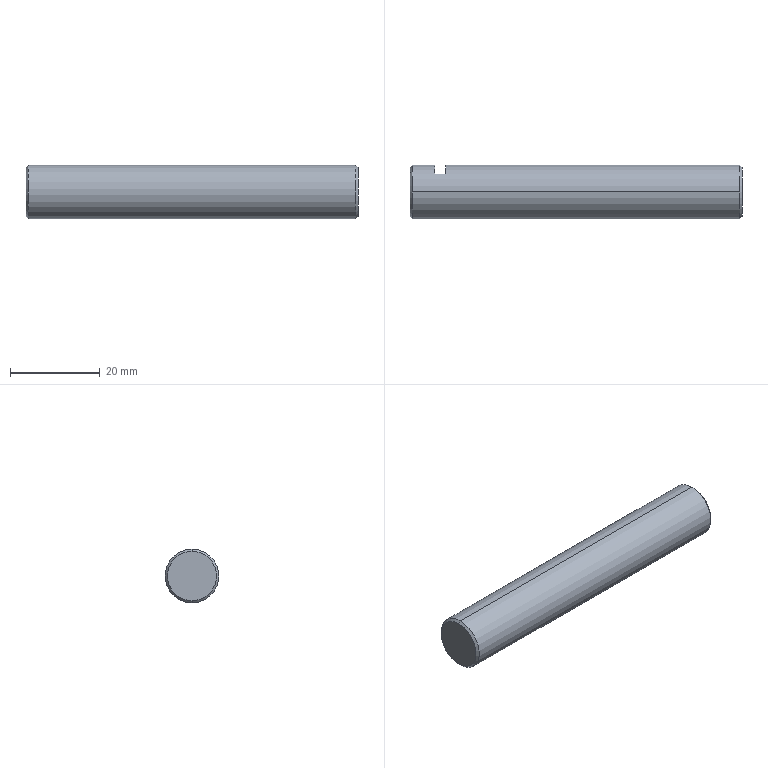Part | STEP file | 0245_010_PCLKG12-74 | 1 solid | 11 faces | box 74 x 12 x 12 mm | volume 8329 mm3 | plane 5 | cone 4 | cylinder 2 | commonest cylinder face diameters 12 x2
STEP:
#1=CARTESIAN_POINT('',(0.,0.,0.));
#2=DIRECTION('',(0.,0.,1.));
#3=DIRECTION('',(1.,0.,0.));
#4=AXIS2_PLACEMENT_3D('',#1,#2,#3);
#5=CARTESIAN_POINT('',(5.5,4.,-4.472));
#6=VERTEX_POINT('',#5);
#7=CARTESIAN_POINT('',(8.,4.,-4.472));
#8=VERTEX_POINT('',#7);
#9=CARTESIAN_POINT('',(37.,4.,-4.472));
#10=DIRECTION('',(1.,0.,0.));
#11=VECTOR('',#10,1.);
#12=LINE('',#9,#11);
#13=CARTESIAN_POINT('',(37.,0.,0.));
#14=DIRECTION('',(1.,0.,0.));
#15=DIRECTION('',(0.,0.,-1.));
#16=AXIS2_PLACEMENT_3D('',#13,#14,#15);
#17=CYLINDRICAL_SURFACE('',#16,6.);
#18=CARTESIAN_POINT('',(0.7297,0.));
#19=DIRECTION('',(0.,1.));
#20=VECTOR('',#19,1.);
#21=LINE('',#18,#20);
#22=(GEOMETRIC_REPRESENTATION_CONTEXT(2)PARAMETRIC_REPRESENTATION_CONTEXT()REPRESENTATION_CONTEXT('',''));
#23=DEFINITIONAL_REPRESENTATION('',(#21),#22);
#24=PCURVE('',#17,#23);
#25=CARTESIAN_POINT('',(5.5,4.,12.));
#26=DIRECTION('',(0.,-1.,0.));
#27=DIRECTION('',(0.,0.,-1.));
#28=AXIS2_PLACEMENT_3D('',#25,#26,#27);
#29=PLANE('',#28);
#30=CARTESIAN_POINT('',(16.472,31.5));
#31=DIRECTION('',(0.,1.));
#32=VECTOR('',#31,1.);
#33=LINE('',#30,#32);
#34=(GEOMETRIC_REPRESENTATION_CONTEXT(2)PARAMETRIC_REPRESENTATION_CONTEXT()REPRESENTATION_CONTEXT('',''));
#35=DEFINITIONAL_REPRESENTATION('',(#33),#34);
#36=PCURVE('',#29,#35);
#37=SURFACE_CURVE('',#12,(#24,#36),.PCURVE_S1.);
#38=EDGE_CURVE('',#6,#8,#37,.T.);
#39=ORIENTED_EDGE('',*,*,#38,.T.);
#40=CARTESIAN_POINT('',(8.,4.,4.472));
#41=VERTEX_POINT('',#40);
#42=CARTESIAN_POINT('',(8.,0.,0.));
#43=DIRECTION('',(1.,0.,0.));
#44=DIRECTION('',(0.,0.,-1.));
#45=AXIS2_PLACEMENT_3D('',#42,#43,#44);
#46=CIRCLE('',#45,6.);
#47=CARTESIAN_POINT('',(0.,-29.));
#48=DIRECTION('',(1.,0.));
#49=VECTOR('',#48,1.);
#50=LINE('',#47,#49);
#51=(GEOMETRIC_REPRESENTATION_CONTEXT(2)PARAMETRIC_REPRESENTATION_CONTEXT()REPRESENTATION_CONTEXT('',''));
#52=DEFINITIONAL_REPRESENTATION('',(#50),#51);
#53=PCURVE('',#17,#52);
#54=CARTESIAN_POINT('',(8.,4.,12.));
#55=DIRECTION('',(1.,0.,0.));
#56=DIRECTION('',(0.,0.,-1.));
#57=AXIS2_PLACEMENT_3D('',#54,#55,#56);
#58=PLANE('',#57);
#59=CARTESIAN_POINT('',(12.,-4.));
#60=DIRECTION('',(1.,0.));
#61=AXIS2_PLACEMENT_2D('',#59,#60);
#62=CIRCLE('',#61,6.);
#63=(GEOMETRIC_REPRESENTATION_CONTEXT(2)PARAMETRIC_REPRESENTATION_CONTEXT()REPRESENTATION_CONTEXT('',''));
#64=DEFINITIONAL_REPRESENTATION('',(#62),#63);
#65=PCURVE('',#58,#64);
#66=SURFACE_CURVE('',#46,(#53,#65),.PCURVE_S1.);
#67=EDGE_CURVE('',#8,#41,#66,.T.);
#68=ORIENTED_EDGE('',*,*,#67,.T.);
#69=CARTESIAN_POINT('',(5.5,4.,4.472));
#70=VERTEX_POINT('',#69);
#71=CARTESIAN_POINT('',(5.5,4.,4.472));
#72=DIRECTION('',(-1.,0.,0.));
#73=VECTOR('',#72,1.);
#74=LINE('',#71,#73);
#75=CARTESIAN_POINT('',(2.412,-31.5));
#76=DIRECTION('',(0.,-1.));
#77=VECTOR('',#76,1.);
#78=LINE('',#75,#77);
#79=(GEOMETRIC_REPRESENTATION_CONTEXT(2)PARAMETRIC_REPRESENTATION_CONTEXT()REPRESENTATION_CONTEXT('',''));
#80=DEFINITIONAL_REPRESENTATION('',(#78),#79);
#81=PCURVE('',#17,#80);
#82=CARTESIAN_POINT('',(7.528,0.));
#83=DIRECTION('',(0.,-1.));
#84=VECTOR('',#83,1.);
#85=LINE('',#82,#84);
#86=(GEOMETRIC_REPRESENTATION_CONTEXT(2)PARAMETRIC_REPRESENTATION_CONTEXT()REPRESENTATION_CONTEXT('',''));
#87=DEFINITIONAL_REPRESENTATION('',(#85),#86);
#88=PCURVE('',#29,#87);
#89=SURFACE_CURVE('',#74,(#81,#88),.PCURVE_S1.);
#90=EDGE_CURVE('',#41,#70,#89,.T.);
#91=ORIENTED_EDGE('',*,*,#90,.T.);
#92=CARTESIAN_POINT('',(5.5,0.,0.));
#93=DIRECTION('',(-1.,0.,0.));
#94=DIRECTION('',(0.,0.,-1.));
#95=AXIS2_PLACEMENT_3D('',#92,#93,#94);
#96=CIRCLE('',#95,6.);
#97=CARTESIAN_POINT('',(6.283,-31.5));
#98=DIRECTION('',(-1.,0.));
#99=VECTOR('',#98,1.);
#100=LINE('',#97,#99);
#101=(GEOMETRIC_REPRESENTATION_CONTEXT(2)PARAMETRIC_REPRESENTATION_CONTEXT()REPRESENTATION_CONTEXT('',''));
#102=DEFINITIONAL_REPRESENTATION('',(#100),#101);
#103=PCURVE('',#17,#102);
#104=CARTESIAN_POINT('',(5.5,8.,12.));
#105=DIRECTION('',(-1.,0.,0.));
#106=DIRECTION('',(0.,0.,1.));
#107=AXIS2_PLACEMENT_3D('',#104,#105,#106);
#108=PLANE('',#107);
#109=CARTESIAN_POINT('',(-12.,-8.));
#110=DIRECTION('',(-1.,0.));
#111=AXIS2_PLACEMENT_2D('',#109,#110);
#112=CIRCLE('',#111,6.);
#113=(GEOMETRIC_REPRESENTATION_CONTEXT(2)PARAMETRIC_REPRESENTATION_CONTEXT()REPRESENTATION_CONTEXT('',''));
#114=DEFINITIONAL_REPRESENTATION('',(#112),#113);
#115=PCURVE('',#108,#114);
#116=SURFACE_CURVE('',#96,(#103,#115),.PCURVE_S1.);
#117=EDGE_CURVE('',#70,#6,#116,.T.);
#118=ORIENTED_EDGE('',*,*,#117,.T.);
#119=EDGE_LOOP('',(#39,#68,#91,#118));
#120=FACE_BOUND('',#119,.T.);
#121=CARTESIAN_POINT('',(0.5,0.,-6.));
#122=VERTEX_POINT('',#121);
#123=CARTESIAN_POINT('',(0.5,0.,6.));
#124=VERTEX_POINT('',#123);
#125=CARTESIAN_POINT('',(0.5,0.,0.));
#126=DIRECTION('',(1.,0.,0.));
#127=DIRECTION('',(0.,0.,-1.));
#128=AXIS2_PLACEMENT_3D('',#125,#126,#127);
#129=CIRCLE('',#128,6.);
#130=CARTESIAN_POINT('',(0.,-36.5));
#131=DIRECTION('',(1.,0.));
#132=VECTOR('',#131,1.);
#133=LINE('',#130,#132);
#134=(GEOMETRIC_REPRESENTATION_CONTEXT(2)PARAMETRIC_REPRESENTATION_CONTEXT()REPRESENTATION_CONTEXT('',''));
#135=DEFINITIONAL_REPRESENTATION('',(#133),#134);
#136=PCURVE('',#17,#135);
#137=CARTESIAN_POINT('',(0.5,0.,0.));
#138=DIRECTION('',(1.,0.,0.));
#139=DIRECTION('',(0.,0.,-1.));
#140=AXIS2_PLACEMENT_3D('',#137,#138,#139);
#141=CONICAL_SURFACE('',#140,6.,0.7854);
#142=CARTESIAN_POINT('',(0.,0.));
#143=DIRECTION('',(1.,0.));
#144=VECTOR('',#143,1.);
#145=LINE('',#142,#144);
#146=(GEOMETRIC_REPRESENTATION_CONTEXT(2)PARAMETRIC_REPRESENTATION_CONTEXT()REPRESENTATION_CONTEXT('',''));
#147=DEFINITIONAL_REPRESENTATION('',(#145),#146);
#148=PCURVE('',#141,#147);
#149=SURFACE_CURVE('',#129,(#136,#148),.PCURVE_S1.);
#150=EDGE_CURVE('',#122,#124,#149,.T.);
#151=ORIENTED_EDGE('',*,*,#150,.T.);
#152=CARTESIAN_POINT('',(73.5,0.,6.));
#153=VERTEX_POINT('',#152);
#154=CARTESIAN_POINT('',(37.,0.,6.));
#155=DIRECTION('',(1.,0.,0.));
#156=VECTOR('',#155,1.);
#157=LINE('',#154,#156);
#158=CARTESIAN_POINT('',(3.142,0.));
#159=DIRECTION('',(0.,1.));
#160=VECTOR('',#159,1.);
#161=LINE('',#158,#160);
#162=(GEOMETRIC_REPRESENTATION_CONTEXT(2)PARAMETRIC_REPRESENTATION_CONTEXT()REPRESENTATION_CONTEXT('',''));
#163=DEFINITIONAL_REPRESENTATION('',(#161),#162);
#164=PCURVE('',#17,#163);
#165=CARTESIAN_POINT('',(37.,0.,0.));
#166=DIRECTION('',(1.,0.,0.));
#167=DIRECTION('',(0.,0.,-1.));
#168=AXIS2_PLACEMENT_3D('',#165,#166,#167);
#169=CYLINDRICAL_SURFACE('',#168,6.);
#170=CARTESIAN_POINT('',(3.142,0.));
#171=DIRECTION('',(0.,1.));
#172=VECTOR('',#171,1.);
#173=LINE('',#170,#172);
#174=(GEOMETRIC_REPRESENTATION_CONTEXT(2)PARAMETRIC_REPRESENTATION_CONTEXT()REPRESENTATION_CONTEXT('',''));
#175=DEFINITIONAL_REPRESENTATION('',(#173),#174);
#176=PCURVE('',#169,#175);
#177=SURFACE_CURVE('',#157,(#164,#176),.PCURVE_S1.);
#178=EDGE_CURVE('',#124,#153,#177,.T.);
#179=ORIENTED_EDGE('',*,*,#178,.T.);
#180=CARTESIAN_POINT('',(73.5,0.,-6.));
#181=VERTEX_POINT('',#180);
#182=CARTESIAN_POINT('',(73.5,0.,0.));
#183=DIRECTION('',(-1.,0.,0.));
#184=DIRECTION('',(0.,0.,-1.));
#185=AXIS2_PLACEMENT_3D('',#182,#183,#184);
#186=CIRCLE('',#185,6.);
#187=CARTESIAN_POINT('',(6.283,36.5));
#188=DIRECTION('',(-1.,0.));
#189=VECTOR('',#188,1.);
#190=LINE('',#187,#189);
#191=(GEOMETRIC_REPRESENTATION_CONTEXT(2)PARAMETRIC_REPRESENTATION_CONTEXT()REPRESENTATION_CONTEXT('',''));
#192=DEFINITIONAL_REPRESENTATION('',(#190),#191);
#193=PCURVE('',#17,#192);
#194=CARTESIAN_POINT('',(73.5,0.,0.));
#195=DIRECTION('',(-1.,0.,0.));
#196=DIRECTION('',(0.,0.,1.));
#197=AXIS2_PLACEMENT_3D('',#194,#195,#196);
#198=CONICAL_SURFACE('',#197,6.,0.7854);
#199=CARTESIAN_POINT('',(-3.142,0.));
#200=DIRECTION('',(1.,0.));
#201=VECTOR('',#200,1.);
#202=LINE('',#199,#201);
#203=(GEOMETRIC_REPRESENTATION_CONTEXT(2)PARAMETRIC_REPRESENTATION_CONTEXT()REPRESENTATION_CONTEXT('',''));
#204=DEFINITIONAL_REPRESENTATION('',(#202),#203);
#205=PCURVE('',#198,#204);
#206=SURFACE_CURVE('',#186,(#193,#205),.PCURVE_S1.);
#207=EDGE_CURVE('',#153,#181,#206,.T.);
#208=ORIENTED_EDGE('',*,*,#207,.T.);
#209=CARTESIAN_POINT('',(37.,0.,-6.));
#210=DIRECTION('',(1.,0.,0.));
#211=VECTOR('',#210,1.);
#212=LINE('',#209,#211);
#213=CARTESIAN_POINT('',(0.,0.));
#214=DIRECTION('',(0.,1.));
#215=VECTOR('',#214,1.);
#216=LINE('',#213,#215);
#217=(GEOMETRIC_REPRESENTATION_CONTEXT(2)PARAMETRIC_REPRESENTATION_CONTEXT()REPRESENTATION_CONTEXT('',''));
#218=DEFINITIONAL_REPRESENTATION('',(#216),#217);
#219=PCURVE('',#17,#218);
#220=CARTESIAN_POINT('',(6.283,0.));
#221=DIRECTION('',(0.,1.));
#222=VECTOR('',#221,1.);
#223=LINE('',#220,#222);
#224=(GEOMETRIC_REPRESENTATION_CONTEXT(2)PARAMETRIC_REPRESENTATION_CONTEXT()REPRESENTATION_CONTEXT('',''));
#225=DEFINITIONAL_REPRESENTATION('',(#223),#224);
#226=PCURVE('',#169,#225);
#227=SURFACE_CURVE('',#212,(#219,#226),.PCURVE_S1.);
#228=EDGE_CURVE('',#122,#181,#227,.T.);
#229=ORIENTED_EDGE('',*,*,#228,.F.);
#230=EDGE_LOOP('',(#151,#179,#208,#229));
#231=FACE_BOUND('',#230,.T.);
#232=ADVANCED_FACE('',(#120,#231),#17,.T.);
#233=CARTESIAN_POINT('',(0.,0.,-5.5));
#234=VERTEX_POINT('',#233);
#235=CARTESIAN_POINT('',(0.,0.,5.5));
#236=VERTEX_POINT('',#235);
#237=CARTESIAN_POINT('',(0.,0.,0.));
#238=DIRECTION('',(1.,0.,0.));
#239=DIRECTION('',(0.,0.,-1.));
#240=AXIS2_PLACEMENT_3D('',#237,#238,#239);
#241=CIRCLE('',#240,5.5);
#242=CARTESIAN_POINT('',(0.,-0.5));
#243=DIRECTION('',(1.,0.));
#244=VECTOR('',#243,1.);
#245=LINE('',#242,#244);
#246=(GEOMETRIC_REPRESENTATION_CONTEXT(2)PARAMETRIC_REPRESENTATION_CONTEXT()REPRESENTATION_CONTEXT('',''));
#247=DEFINITIONAL_REPRESENTATION('',(#245),#246);
#248=PCURVE('',#141,#247);
#249=CARTESIAN_POINT('',(0.,2.75,0.));
#250=DIRECTION('',(-1.,0.,0.));
#251=DIRECTION('',(0.,0.,1.));
#252=AXIS2_PLACEMENT_3D('',#249,#250,#251);
#253=PLANE('',#252);
#254=CARTESIAN_POINT('',(-5.5,-2.75));
#255=CARTESIAN_POINT('',(-5.5,6.776));
#256=CARTESIAN_POINT('',(2.75,2.013));
#257=CARTESIAN_POINT('',(11.,-2.75));
#258=CARTESIAN_POINT('',(2.75,-7.513));
#259=CARTESIAN_POINT('',(-5.5,-12.276));
#260=CARTESIAN_POINT('',(-5.5,-2.75));
#261=(BOUNDED_CURVE()B_SPLINE_CURVE(2,(#254,#255,#256,#257,#258,#259,#260),.UNSPECIFIED.,.T.,.F.)B_SPLINE_CURVE_WITH_KNOTS((1,2,2,2,2,1),(-2.094,0.,2.094,4.189,6.283,8.378),.UNSPECIFIED.)CURVE()GEOMETRIC_REPRESENTATION_ITEM()RATIONAL_B_SPLINE_CURVE((1.,0.5,1.,0.5,1.,0.5,1.))REPRESENTATION_ITEM(''));
#262=(GEOMETRIC_REPRESENTATION_CONTEXT(2)PARAMETRIC_REPRESENTATION_CONTEXT()REPRESENTATION_CONTEXT('',''));
#263=DEFINITIONAL_REPRESENTATION('',(#261),#262);
#264=PCURVE('',#253,#263);
#265=SURFACE_CURVE('',#241,(#248,#264),.PCURVE_S1.);
#266=EDGE_CURVE('',#234,#236,#265,.T.);
#267=ORIENTED_EDGE('',*,*,#266,.T.);
#268=CARTESIAN_POINT('',(0.5,0.,6.));
#269=DIRECTION('',(0.7071,0.,0.7071));
#270=VECTOR('',#269,1.);
#271=LINE('',#268,#270);
#272=CARTESIAN_POINT('',(3.142,0.));
#273=DIRECTION('',(0.,1.));
#274=VECTOR('',#273,1.);
#275=LINE('',#272,#274);
#276=(GEOMETRIC_REPRESENTATION_CONTEXT(2)PARAMETRIC_REPRESENTATION_CONTEXT()REPRESENTATION_CONTEXT('',''));
#277=DEFINITIONAL_REPRESENTATION('',(#275),#276);
#278=PCURVE('',#141,#277);
#279=CARTESIAN_POINT('',(0.5,0.,0.));
#280=DIRECTION('',(1.,0.,0.));
#281=DIRECTION('',(0.,0.,-1.));
#282=AXIS2_PLACEMENT_3D('',#279,#280,#281);
#283=CONICAL_SURFACE('',#282,6.,0.7854);
#284=CARTESIAN_POINT('',(3.142,0.));
#285=DIRECTION('',(0.,1.));
#286=VECTOR('',#285,1.);
#287=LINE('',#284,#286);
#288=(GEOMETRIC_REPRESENTATION_CONTEXT(2)PARAMETRIC_REPRESENTATION_CONTEXT()REPRESENTATION_CONTEXT('',''));
#289=DEFINITIONAL_REPRESENTATION('',(#287),#288);
#290=PCURVE('',#283,#289);
#291=SURFACE_CURVE('',#271,(#278,#290),.PCURVE_S1.);
#292=EDGE_CURVE('',#236,#124,#291,.T.);
#293=ORIENTED_EDGE('',*,*,#292,.T.);
#294=ORIENTED_EDGE('',*,*,#150,.F.);
#295=CARTESIAN_POINT('',(0.5,0.,-6.));
#296=DIRECTION('',(0.7071,0.,-0.7071));
#297=VECTOR('',#296,1.);
#298=LINE('',#295,#297);
#299=CARTESIAN_POINT('',(0.,0.));
#300=DIRECTION('',(0.,1.));
#301=VECTOR('',#300,1.);
#302=LINE('',#299,#301);
#303=(GEOMETRIC_REPRESENTATION_CONTEXT(2)PARAMETRIC_REPRESENTATION_CONTEXT()REPRESENTATION_CONTEXT('',''));
#304=DEFINITIONAL_REPRESENTATION('',(#302),#303);
#305=PCURVE('',#141,#304);
#306=CARTESIAN_POINT('',(6.283,0.));
#307=DIRECTION('',(0.,1.));
#308=VECTOR('',#307,1.);
#309=LINE('',#306,#308);
#310=(GEOMETRIC_REPRESENTATION_CONTEXT(2)PARAMETRIC_REPRESENTATION_CONTEXT()REPRESENTATION_CONTEXT('',''));
#311=DEFINITIONAL_REPRESENTATION('',(#309),#310);
#312=PCURVE('',#283,#311);
#313=SURFACE_CURVE('',#298,(#305,#312),.PCURVE_S1.);
#314=EDGE_CURVE('',#234,#122,#313,.T.);
#315=ORIENTED_EDGE('',*,*,#314,.F.);
#316=EDGE_LOOP('',(#267,#293,#294,#315));
#317=FACE_BOUND('',#316,.T.);
#318=ADVANCED_FACE('',(#317),#141,.T.);
#319=CARTESIAN_POINT('',(74.,0.,5.5));
#320=VERTEX_POINT('',#319);
#321=CARTESIAN_POINT('',(74.,0.,-5.5));
#322=VERTEX_POINT('',#321);
#323=CARTESIAN_POINT('',(74.,0.,0.));
#324=DIRECTION('',(-1.,0.,0.));
#325=DIRECTION('',(0.,0.,1.));
#326=AXIS2_PLACEMENT_3D('',#323,#324,#325);
#327=CIRCLE('',#326,5.5);
#328=CARTESIAN_POINT('',(0.,-0.5));
#329=DIRECTION('',(1.,0.));
#330=VECTOR('',#329,1.);
#331=LINE('',#328,#330);
#332=(GEOMETRIC_REPRESENTATION_CONTEXT(2)PARAMETRIC_REPRESENTATION_CONTEXT()REPRESENTATION_CONTEXT('',''));
#333=DEFINITIONAL_REPRESENTATION('',(#331),#332);
#334=PCURVE('',#198,#333);
#335=CARTESIAN_POINT('',(74.,2.75,0.));
#336=DIRECTION('',(1.,0.,0.));
#337=DIRECTION('',(0.,0.,-1.));
#338=AXIS2_PLACEMENT_3D('',#335,#336,#337);
#339=PLANE('',#338);
#340=CARTESIAN_POINT('',(-5.5,-2.75));
#341=CARTESIAN_POINT('',(-5.5,6.776));
#342=CARTESIAN_POINT('',(2.75,2.013));
#343=CARTESIAN_POINT('',(11.,-2.75));
#344=CARTESIAN_POINT('',(2.75,-7.513));
#345=CARTESIAN_POINT('',(-5.5,-12.276));
#346=CARTESIAN_POINT('',(-5.5,-2.75));
#347=(BOUNDED_CURVE()B_SPLINE_CURVE(2,(#340,#341,#342,#343,#344,#345,#346),.UNSPECIFIED.,.T.,.F.)B_SPLINE_CURVE_WITH_KNOTS((1,2,2,2,2,1),(-2.094,0.,2.094,4.189,6.283,8.378),.UNSPECIFIED.)CURVE()GEOMETRIC_REPRESENTATION_ITEM()RATIONAL_B_SPLINE_CURVE((1.,0.5,1.,0.5,1.,0.5,1.))REPRESENTATION_ITEM(''));
#348=(GEOMETRIC_REPRESENTATION_CONTEXT(2)PARAMETRIC_REPRESENTATION_CONTEXT()REPRESENTATION_CONTEXT('',''));
#349=DEFINITIONAL_REPRESENTATION('',(#347),#348);
#350=PCURVE('',#339,#349);
#351=SURFACE_CURVE('',#327,(#334,#350),.PCURVE_S1.);
#352=EDGE_CURVE('',#320,#322,#351,.T.);
#353=ORIENTED_EDGE('',*,*,#352,.T.);
#354=CARTESIAN_POINT('',(73.5,0.,-6.));
#355=DIRECTION('',(-0.7071,0.,-0.7071));
#356=VECTOR('',#355,1.);
#357=LINE('',#354,#356);
#358=CARTESIAN_POINT('',(3.142,0.));
#359=DIRECTION('',(0.,1.));
#360=VECTOR('',#359,1.);
#361=LINE('',#358,#360);
#362=(GEOMETRIC_REPRESENTATION_CONTEXT(2)PARAMETRIC_REPRESENTATION_CONTEXT()REPRESENTATION_CONTEXT('',''));
#363=DEFINITIONAL_REPRESENTATION('',(#361),#362);
#364=PCURVE('',#198,#363);
#365=CARTESIAN_POINT('',(73.5,0.,0.));
#366=DIRECTION('',(-1.,0.,0.));
#367=DIRECTION('',(0.,0.,1.));
#368=AXIS2_PLACEMENT_3D('',#365,#366,#367);
#369=CONICAL_SURFACE('',#368,6.,0.7854);
#370=CARTESIAN_POINT('',(3.142,0.));
#371=DIRECTION('',(0.,1.));
#372=VECTOR('',#371,1.);
#373=LINE('',#370,#372);
#374=(GEOMETRIC_REPRESENTATION_CONTEXT(2)PARAMETRIC_REPRESENTATION_CONTEXT()REPRESENTATION_CONTEXT('',''));
#375=DEFINITIONAL_REPRESENTATION('',(#373),#374);
#376=PCURVE('',#369,#375);
#377=SURFACE_CURVE('',#357,(#364,#376),.PCURVE_S1.);
#378=EDGE_CURVE('',#322,#181,#377,.T.);
#379=ORIENTED_EDGE('',*,*,#378,.T.);
#380=ORIENTED_EDGE('',*,*,#207,.F.);
#381=CARTESIAN_POINT('',(73.5,0.,6.));
#382=DIRECTION('',(-0.7071,0.,0.7071));
#383=VECTOR('',#382,1.);
#384=LINE('',#381,#383);
#385=CARTESIAN_POINT('',(0.,0.));
#386=DIRECTION('',(0.,1.));
#387=VECTOR('',#386,1.);
#388=LINE('',#385,#387);
#389=(GEOMETRIC_REPRESENTATION_CONTEXT(2)PARAMETRIC_REPRESENTATION_CONTEXT()REPRESENTATION_CONTEXT('',''));
#390=DEFINITIONAL_REPRESENTATION('',(#388),#389);
#391=PCURVE('',#198,#390);
#392=CARTESIAN_POINT('',(6.283,0.));
#393=DIRECTION('',(0.,1.));
#394=VECTOR('',#393,1.);
#395=LINE('',#392,#394);
#396=(GEOMETRIC_REPRESENTATION_CONTEXT(2)PARAMETRIC_REPRESENTATION_CONTEXT()REPRESENTATION_CONTEXT('',''));
#397=DEFINITIONAL_REPRESENTATION('',(#395),#396);
#398=PCURVE('',#369,#397);
#399=SURFACE_CURVE('',#384,(#391,#398),.PCURVE_S1.);
#400=EDGE_CURVE('',#320,#153,#399,.T.);
#401=ORIENTED_EDGE('',*,*,#400,.F.);
#402=EDGE_LOOP('',(#353,#379,#380,#401));
#403=FACE_BOUND('',#402,.T.);
#404=ADVANCED_FACE('',(#403),#198,.T.);
#405=ORIENTED_EDGE('',*,*,#178,.F.);
#406=CARTESIAN_POINT('',(0.5,0.,0.));
#407=DIRECTION('',(1.,0.,0.));
#408=DIRECTION('',(0.,0.,-1.));
#409=AXIS2_PLACEMENT_3D('',#406,#407,#408);
#410=CIRCLE('',#409,6.);
#411=CARTESIAN_POINT('',(0.,-36.5));
#412=DIRECTION('',(1.,0.));
#413=VECTOR('',#412,1.);
#414=LINE('',#411,#413);
#415=(GEOMETRIC_REPRESENTATION_CONTEXT(2)PARAMETRIC_REPRESENTATION_CONTEXT()REPRESENTATION_CONTEXT('',''));
#416=DEFINITIONAL_REPRESENTATION('',(#414),#415);
#417=PCURVE('',#169,#416);
#418=CARTESIAN_POINT('',(0.,0.));
#419=DIRECTION('',(1.,0.));
#420=VECTOR('',#419,1.);
#421=LINE('',#418,#420);
#422=(GEOMETRIC_REPRESENTATION_CONTEXT(2)PARAMETRIC_REPRESENTATION_CONTEXT()REPRESENTATION_CONTEXT('',''));
#423=DEFINITIONAL_REPRESENTATION('',(#421),#422);
#424=PCURVE('',#283,#423);
#425=SURFACE_CURVE('',#410,(#417,#424),.PCURVE_S1.);
#426=EDGE_CURVE('',#124,#122,#425,.T.);
#427=ORIENTED_EDGE('',*,*,#426,.T.);
#428=ORIENTED_EDGE('',*,*,#228,.T.);
#429=CARTESIAN_POINT('',(73.5,0.,0.));
#430=DIRECTION('',(-1.,0.,0.));
#431=DIRECTION('',(0.,0.,-1.));
#432=AXIS2_PLACEMENT_3D('',#429,#430,#431);
#433=CIRCLE('',#432,6.);
#434=CARTESIAN_POINT('',(6.283,36.5));
#435=DIRECTION('',(-1.,0.));
#436=VECTOR('',#435,1.);
#437=LINE('',#434,#436);
#438=(GEOMETRIC_REPRESENTATION_CONTEXT(2)PARAMETRIC_REPRESENTATION_CONTEXT()REPRESENTATION_CONTEXT('',''));
#439=DEFINITIONAL_REPRESENTATION('',(#437),#438);
#440=PCURVE('',#169,#439);
#441=CARTESIAN_POINT('',(3.142,0.));
#442=DIRECTION('',(1.,0.));
#443=VECTOR('',#442,1.);
#444=LINE('',#441,#443);
#445=(GEOMETRIC_REPRESENTATION_CONTEXT(2)PARAMETRIC_REPRESENTATION_CONTEXT()REPRESENTATION_CONTEXT('',''));
#446=DEFINITIONAL_REPRESENTATION('',(#444),#445);
#447=PCURVE('',#369,#446);
#448=SURFACE_CURVE('',#433,(#440,#447),.PCURVE_S1.);
#449=EDGE_CURVE('',#181,#153,#448,.T.);
#450=ORIENTED_EDGE('',*,*,#449,.T.);
#451=EDGE_LOOP('',(#405,#427,#428,#450));
#452=FACE_BOUND('',#451,.T.);
#453=ADVANCED_FACE('',(#452),#169,.T.);
#454=CARTESIAN_POINT('',(8.,4.,12.));
#455=DIRECTION('',(0.,0.,-1.));
#456=VECTOR('',#455,1.);
#457=LINE('',#454,#456);
#458=CARTESIAN_POINT('',(0.,0.));
#459=DIRECTION('',(1.,0.));
#460=VECTOR('',#459,1.);
#461=LINE('',#458,#460);
#462=(GEOMETRIC_REPRESENTATION_CONTEXT(2)PARAMETRIC_REPRESENTATION_CONTEXT()REPRESENTATION_CONTEXT('',''));
#463=DEFINITIONAL_REPRESENTATION('',(#461),#462);
#464=PCURVE('',#58,#463);
#465=CARTESIAN_POINT('',(0.,2.5));
#466=DIRECTION('',(1.,0.));
#467=VECTOR('',#466,1.);
#468=LINE('',#465,#467);
#469=(GEOMETRIC_REPRESENTATION_CONTEXT(2)PARAMETRIC_REPRESENTATION_CONTEXT()REPRESENTATION_CONTEXT('',''));
#470=DEFINITIONAL_REPRESENTATION('',(#468),#469);
#471=PCURVE('',#29,#470);
#472=SURFACE_CURVE('',#457,(#464,#471),.PCURVE_S1.);
#473=EDGE_CURVE('',#41,#8,#472,.T.);
#474=ORIENTED_EDGE('',*,*,#473,.F.);
#475=ORIENTED_EDGE('',*,*,#67,.F.);
#476=EDGE_LOOP('',(#474,#475));
#477=FACE_BOUND('',#476,.T.);
#478=ADVANCED_FACE('',(#477),#58,.F.);
#479=CARTESIAN_POINT('',(5.5,4.,12.));
#480=DIRECTION('',(0.,0.,-1.));
#481=VECTOR('',#480,1.);
#482=LINE('',#479,#481);
#483=CARTESIAN_POINT('',(0.,0.));
#484=DIRECTION('',(1.,0.));
#485=VECTOR('',#484,1.);
#486=LINE('',#483,#485);
#487=(GEOMETRIC_REPRESENTATION_CONTEXT(2)PARAMETRIC_REPRESENTATION_CONTEXT()REPRESENTATION_CONTEXT('',''));
#488=DEFINITIONAL_REPRESENTATION('',(#486),#487);
#489=PCURVE('',#29,#488);
#490=CARTESIAN_POINT('',(0.,-4.));
#491=DIRECTION('',(-1.,0.));
#492=VECTOR('',#491,1.);
#493=LINE('',#490,#492);
#494=(GEOMETRIC_REPRESENTATION_CONTEXT(2)PARAMETRIC_REPRESENTATION_CONTEXT()REPRESENTATION_CONTEXT('',''));
#495=DEFINITIONAL_REPRESENTATION('',(#493),#494);
#496=PCURVE('',#108,#495);
#497=SURFACE_CURVE('',#482,(#489,#496),.PCURVE_S1.);
#498=EDGE_CURVE('',#70,#6,#497,.T.);
#499=ORIENTED_EDGE('',*,*,#498,.F.);
#500=ORIENTED_EDGE('',*,*,#90,.F.);
#501=ORIENTED_EDGE('',*,*,#473,.T.);
#502=ORIENTED_EDGE('',*,*,#38,.F.);
#503=EDGE_LOOP('',(#499,#500,#501,#502));
#504=FACE_BOUND('',#503,.T.);
#505=ADVANCED_FACE('',(#504),#29,.F.);
#506=ORIENTED_EDGE('',*,*,#498,.T.);
#507=ORIENTED_EDGE('',*,*,#117,.F.);
#508=EDGE_LOOP('',(#506,#507));
#509=FACE_BOUND('',#508,.T.);
#510=ADVANCED_FACE('',(#509),#108,.F.);
#511=ORIENTED_EDGE('',*,*,#292,.F.);
#512=CARTESIAN_POINT('',(0.,0.,0.));
#513=DIRECTION('',(1.,0.,0.));
#514=DIRECTION('',(0.,0.,-1.));
#515=AXIS2_PLACEMENT_3D('',#512,#513,#514);
#516=CIRCLE('',#515,5.5);
#517=CARTESIAN_POINT('',(0.,-0.5));
#518=DIRECTION('',(1.,0.));
#519=VECTOR('',#518,1.);
#520=LINE('',#517,#519);
#521=(GEOMETRIC_REPRESENTATION_CONTEXT(2)PARAMETRIC_REPRESENTATION_CONTEXT()REPRESENTATION_CONTEXT('',''));
#522=DEFINITIONAL_REPRESENTATION('',(#520),#521);
#523=PCURVE('',#283,#522);
#524=CARTESIAN_POINT('',(-5.5,-2.75));
#525=CARTESIAN_POINT('',(-5.5,6.776));
#526=CARTESIAN_POINT('',(2.75,2.013));
#527=CARTESIAN_POINT('',(11.,-2.75));
#528=CARTESIAN_POINT('',(2.75,-7.513));
#529=CARTESIAN_POINT('',(-5.5,-12.276));
#530=CARTESIAN_POINT('',(-5.5,-2.75));
#531=(BOUNDED_CURVE()B_SPLINE_CURVE(2,(#524,#525,#526,#527,#528,#529,#530),.UNSPECIFIED.,.T.,.F.)B_SPLINE_CURVE_WITH_KNOTS((1,2,2,2,2,1),(-2.094,0.,2.094,4.189,6.283,8.378),.UNSPECIFIED.)CURVE()GEOMETRIC_REPRESENTATION_ITEM()RATIONAL_B_SPLINE_CURVE((1.,0.5,1.,0.5,1.,0.5,1.))REPRESENTATION_ITEM(''));
#532=(GEOMETRIC_REPRESENTATION_CONTEXT(2)PARAMETRIC_REPRESENTATION_CONTEXT()REPRESENTATION_CONTEXT('',''));
#533=DEFINITIONAL_REPRESENTATION('',(#531),#532);
#534=PCURVE('',#253,#533);
#535=SURFACE_CURVE('',#516,(#523,#534),.PCURVE_S1.);
#536=EDGE_CURVE('',#236,#234,#535,.T.);
#537=ORIENTED_EDGE('',*,*,#536,.T.);
#538=ORIENTED_EDGE('',*,*,#314,.T.);
#539=ORIENTED_EDGE('',*,*,#426,.F.);
#540=EDGE_LOOP('',(#511,#537,#538,#539));
#541=FACE_BOUND('',#540,.T.);
#542=ADVANCED_FACE('',(#541),#283,.T.);
#543=ORIENTED_EDGE('',*,*,#378,.F.);
#544=CARTESIAN_POINT('',(74.,0.,0.));
#545=DIRECTION('',(-1.,0.,0.));
#546=DIRECTION('',(0.,0.,1.));
#547=AXIS2_PLACEMENT_3D('',#544,#545,#546);
#548=CIRCLE('',#547,5.5);
#549=CARTESIAN_POINT('',(0.,-0.5));
#550=DIRECTION('',(1.,0.));
#551=VECTOR('',#550,1.);
#552=LINE('',#549,#551);
#553=(GEOMETRIC_REPRESENTATION_CONTEXT(2)PARAMETRIC_REPRESENTATION_CONTEXT()REPRESENTATION_CONTEXT('',''));
#554=DEFINITIONAL_REPRESENTATION('',(#552),#553);
#555=PCURVE('',#369,#554);
#556=CARTESIAN_POINT('',(-5.5,-2.75));
#557=CARTESIAN_POINT('',(-5.5,6.776));
#558=CARTESIAN_POINT('',(2.75,2.013));
#559=CARTESIAN_POINT('',(11.,-2.75));
#560=CARTESIAN_POINT('',(2.75,-7.513));
#561=CARTESIAN_POINT('',(-5.5,-12.276));
#562=CARTESIAN_POINT('',(-5.5,-2.75));
#563=(BOUNDED_CURVE()B_SPLINE_CURVE(2,(#556,#557,#558,#559,#560,#561,#562),.UNSPECIFIED.,.T.,.F.)B_SPLINE_CURVE_WITH_KNOTS((1,2,2,2,2,1),(-2.094,0.,2.094,4.189,6.283,8.378),.UNSPECIFIED.)CURVE()GEOMETRIC_REPRESENTATION_ITEM()RATIONAL_B_SPLINE_CURVE((1.,0.5,1.,0.5,1.,0.5,1.))REPRESENTATION_ITEM(''));
#564=(GEOMETRIC_REPRESENTATION_CONTEXT(2)PARAMETRIC_REPRESENTATION_CONTEXT()REPRESENTATION_CONTEXT('',''));
#565=DEFINITIONAL_REPRESENTATION('',(#563),#564);
#566=PCURVE('',#339,#565);
#567=SURFACE_CURVE('',#548,(#555,#566),.PCURVE_S1.);
#568=EDGE_CURVE('',#322,#320,#567,.T.);
#569=ORIENTED_EDGE('',*,*,#568,.T.);
#570=ORIENTED_EDGE('',*,*,#400,.T.);
#571=ORIENTED_EDGE('',*,*,#449,.F.);
#572=EDGE_LOOP('',(#543,#569,#570,#571));
#573=FACE_BOUND('',#572,.T.);
#574=ADVANCED_FACE('',(#573),#369,.T.);
#575=ORIENTED_EDGE('',*,*,#266,.F.);
#576=ORIENTED_EDGE('',*,*,#536,.F.);
#577=EDGE_LOOP('',(#575,#576));
#578=FACE_BOUND('',#577,.T.);
#579=ADVANCED_FACE('',(#578),#253,.T.);
#580=ORIENTED_EDGE('',*,*,#352,.F.);
#581=ORIENTED_EDGE('',*,*,#568,.F.);
#582=EDGE_LOOP('',(#580,#581));
#583=FACE_BOUND('',#582,.T.);
#584=ADVANCED_FACE('',(#583),#339,.T.);
#585=CLOSED_SHELL('',(#232,#318,#404,#453,#478,#505,#510,#542,#574,#579,#584));
#586=MANIFOLD_SOLID_BREP('',#585);
#587=(LENGTH_UNIT()NAMED_UNIT(*)SI_UNIT(.MILLI.,.METRE.));
#588=UNCERTAINTY_MEASURE_WITH_UNIT(LENGTH_MEASURE(0.0000001),#587,'','');
#589=(NAMED_UNIT(*)PLANE_ANGLE_UNIT()SI_UNIT($,.RADIAN.));
#590=(NAMED_UNIT(*)SI_UNIT($,.STERADIAN.)SOLID_ANGLE_UNIT());
#591=(GEOMETRIC_REPRESENTATION_CONTEXT(3)GLOBAL_UNCERTAINTY_ASSIGNED_CONTEXT((#588))GLOBAL_UNIT_ASSIGNED_CONTEXT((#587,#589,#590))REPRESENTATION_CONTEXT('',''));
#592=ADVANCED_BREP_SHAPE_REPRESENTATION('',(#4,#586),#591);